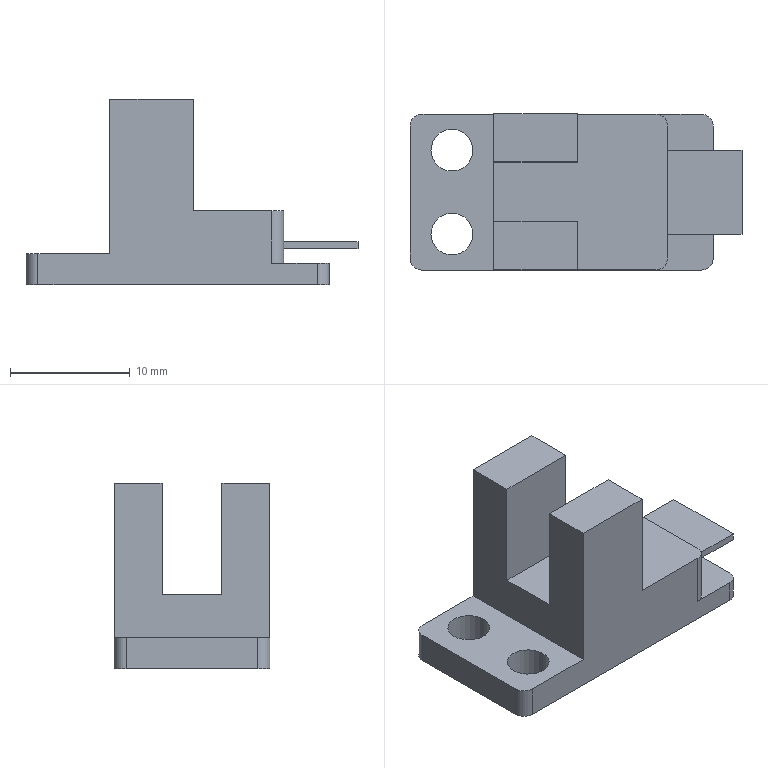Part | NX | 1 solid | 29 faces | box 27.7 x 13 x 15.5 mm | volume 1984 mm3 | plane 21 | cylinder 8 | commonest cylinder face diameters 2 x6 3.5 x2
STEP:
#1=CARTESIAN_POINT('',(5.25,3.,2.6));
#2=VERTEX_POINT('',#1);
#3=CARTESIAN_POINT('',(3.5,3.,2.6));
#4=DIRECTION('',(0.,0.,1.));
#5=DIRECTION('',(1.,0.,0.));
#6=AXIS2_PLACEMENT_3D('',#3,#4,#5);
#7=CIRCLE('',#6,1.75);
#8=EDGE_CURVE('',#2,#2,#7,.T.);
#9=ORIENTED_EDGE('',*,*,#8,.T.);
#10=EDGE_LOOP('',(#9));
#11=FACE_BOUND('',#10,.T.);
#12=CARTESIAN_POINT('',(5.25,3.,0.));
#13=VERTEX_POINT('',#12);
#14=CARTESIAN_POINT('',(3.5,3.,0.));
#15=DIRECTION('',(0.,0.,1.));
#16=DIRECTION('',(1.,0.,0.));
#17=AXIS2_PLACEMENT_3D('',#14,#15,#16);
#18=CIRCLE('',#17,1.75);
#19=EDGE_CURVE('',#13,#13,#18,.F.);
#20=ORIENTED_EDGE('',*,*,#19,.T.);
#21=EDGE_LOOP('',(#20));
#22=FACE_BOUND('',#21,.T.);
#23=CARTESIAN_POINT('',(3.5,3.,0.));
#24=DIRECTION('',(0.,0.,1.));
#25=DIRECTION('',(1.,0.,0.));
#26=AXIS2_PLACEMENT_3D('',#23,#24,#25);
#27=CYLINDRICAL_SURFACE('',#26,1.75);
#28=ADVANCED_FACE('',(#11,#22),#27,.F.);
#29=CARTESIAN_POINT('',(5.25,10.,2.6));
#30=VERTEX_POINT('',#29);
#31=CARTESIAN_POINT('',(3.5,10.,2.6));
#32=DIRECTION('',(0.,0.,1.));
#33=DIRECTION('',(1.,0.,0.));
#34=AXIS2_PLACEMENT_3D('',#31,#32,#33);
#35=CIRCLE('',#34,1.75);
#36=EDGE_CURVE('',#30,#30,#35,.T.);
#37=ORIENTED_EDGE('',*,*,#36,.F.);
#38=EDGE_LOOP('',(#37));
#39=FACE_BOUND('',#38,.T.);
#40=ORIENTED_EDGE('',*,*,#8,.F.);
#41=EDGE_LOOP('',(#40));
#42=FACE_BOUND('',#41,.T.);
#43=CARTESIAN_POINT('',(0.,1.,2.6));
#44=VERTEX_POINT('',#43);
#45=CARTESIAN_POINT('',(1.,0.,2.6));
#46=VERTEX_POINT('',#45);
#47=CARTESIAN_POINT('',(1.,1.,2.6));
#48=DIRECTION('',(0.,0.,-1.));
#49=DIRECTION('',(-1.,0.,0.));
#50=AXIS2_PLACEMENT_3D('',#47,#48,#49);
#51=CIRCLE('',#50,1.);
#52=EDGE_CURVE('',#44,#46,#51,.F.);
#53=ORIENTED_EDGE('',*,*,#52,.T.);
#54=CARTESIAN_POINT('',(7.,0.,2.6));
#55=VERTEX_POINT('',#54);
#56=CARTESIAN_POINT('',(3.5,0.,2.6));
#57=DIRECTION('',(-1.,0.,0.));
#58=VECTOR('',#57,1000.);
#59=LINE('',#56,#58);
#60=EDGE_CURVE('',#55,#46,#59,.T.);
#61=ORIENTED_EDGE('',*,*,#60,.F.);
#62=CARTESIAN_POINT('',(7.,13.,2.6));
#63=VERTEX_POINT('',#62);
#64=CARTESIAN_POINT('',(7.,6.5,2.6));
#65=DIRECTION('',(0.,-1.,0.));
#66=VECTOR('',#65,1000.);
#67=LINE('',#64,#66);
#68=EDGE_CURVE('',#63,#55,#67,.T.);
#69=ORIENTED_EDGE('',*,*,#68,.F.);
#70=CARTESIAN_POINT('',(1.,13.,2.6));
#71=VERTEX_POINT('',#70);
#72=CARTESIAN_POINT('',(3.5,13.,2.6));
#73=DIRECTION('',(1.,0.,0.));
#74=VECTOR('',#73,1000.);
#75=LINE('',#72,#74);
#76=EDGE_CURVE('',#71,#63,#75,.T.);
#77=ORIENTED_EDGE('',*,*,#76,.F.);
#78=CARTESIAN_POINT('',(0.,12.,2.6));
#79=VERTEX_POINT('',#78);
#80=CARTESIAN_POINT('',(1.,12.,2.6));
#81=DIRECTION('',(0.,0.,-1.));
#82=DIRECTION('',(-1.,0.,0.));
#83=AXIS2_PLACEMENT_3D('',#80,#81,#82);
#84=CIRCLE('',#83,1.);
#85=EDGE_CURVE('',#71,#79,#84,.F.);
#86=ORIENTED_EDGE('',*,*,#85,.T.);
#87=CARTESIAN_POINT('',(0.,6.5,2.6));
#88=DIRECTION('',(0.,1.,0.));
#89=VECTOR('',#88,1000.);
#90=LINE('',#87,#89);
#91=EDGE_CURVE('',#44,#79,#90,.T.);
#92=ORIENTED_EDGE('',*,*,#91,.F.);
#93=EDGE_LOOP('',(#53,#61,#69,#77,#86,#92));
#94=FACE_BOUND('',#93,.T.);
#95=CARTESIAN_POINT('',(7.,0.,2.6));
#96=DIRECTION('',(0.,0.,-1.));
#97=DIRECTION('',(-1.,0.,0.));
#98=AXIS2_PLACEMENT_3D('',#95,#96,#97);
#99=PLANE('',#98);
#100=ADVANCED_FACE('',(#39,#42,#94),#99,.F.);
#101=CARTESIAN_POINT('',(5.25,10.,0.));
#102=VERTEX_POINT('',#101);
#103=CARTESIAN_POINT('',(3.5,10.,0.));
#104=DIRECTION('',(0.,0.,1.));
#105=DIRECTION('',(1.,0.,0.));
#106=AXIS2_PLACEMENT_3D('',#103,#104,#105);
#107=CIRCLE('',#106,1.75);
#108=EDGE_CURVE('',#102,#102,#107,.T.);
#109=ORIENTED_EDGE('',*,*,#108,.T.);
#110=EDGE_LOOP('',(#109));
#111=FACE_BOUND('',#110,.T.);
#112=ORIENTED_EDGE('',*,*,#19,.F.);
#113=EDGE_LOOP('',(#112));
#114=FACE_BOUND('',#113,.T.);
#115=CARTESIAN_POINT('',(1.,13.,0.));
#116=VERTEX_POINT('',#115);
#117=CARTESIAN_POINT('',(24.3,13.,0.));
#118=VERTEX_POINT('',#117);
#119=CARTESIAN_POINT('',(12.65,13.,0.));
#120=DIRECTION('',(1.,0.,0.));
#121=VECTOR('',#120,1000.);
#122=LINE('',#119,#121);
#123=EDGE_CURVE('',#116,#118,#122,.T.);
#124=ORIENTED_EDGE('',*,*,#123,.T.);
#125=CARTESIAN_POINT('',(25.3,12.,0.));
#126=VERTEX_POINT('',#125);
#127=CARTESIAN_POINT('',(24.3,12.,0.));
#128=DIRECTION('',(0.,0.,-1.));
#129=DIRECTION('',(-1.,0.,0.));
#130=AXIS2_PLACEMENT_3D('',#127,#128,#129);
#131=CIRCLE('',#130,1.);
#132=EDGE_CURVE('',#118,#126,#131,.T.);
#133=ORIENTED_EDGE('',*,*,#132,.T.);
#134=CARTESIAN_POINT('',(25.3,1.,0.));
#135=VERTEX_POINT('',#134);
#136=CARTESIAN_POINT('',(25.3,6.5,0.));
#137=DIRECTION('',(0.,-1.,0.));
#138=VECTOR('',#137,1000.);
#139=LINE('',#136,#138);
#140=EDGE_CURVE('',#126,#135,#139,.T.);
#141=ORIENTED_EDGE('',*,*,#140,.T.);
#142=CARTESIAN_POINT('',(24.3,0.,0.));
#143=VERTEX_POINT('',#142);
#144=CARTESIAN_POINT('',(24.3,1.,0.));
#145=DIRECTION('',(0.,0.,-1.));
#146=DIRECTION('',(-1.,0.,0.));
#147=AXIS2_PLACEMENT_3D('',#144,#145,#146);
#148=CIRCLE('',#147,1.);
#149=EDGE_CURVE('',#135,#143,#148,.T.);
#150=ORIENTED_EDGE('',*,*,#149,.T.);
#151=CARTESIAN_POINT('',(1.,0.,0.));
#152=VERTEX_POINT('',#151);
#153=CARTESIAN_POINT('',(12.65,0.,0.));
#154=DIRECTION('',(-1.,0.,0.));
#155=VECTOR('',#154,1000.);
#156=LINE('',#153,#155);
#157=EDGE_CURVE('',#143,#152,#156,.T.);
#158=ORIENTED_EDGE('',*,*,#157,.T.);
#159=CARTESIAN_POINT('',(0.,1.,0.));
#160=VERTEX_POINT('',#159);
#161=CARTESIAN_POINT('',(1.,1.,0.));
#162=DIRECTION('',(0.,0.,-1.));
#163=DIRECTION('',(-1.,0.,0.));
#164=AXIS2_PLACEMENT_3D('',#161,#162,#163);
#165=CIRCLE('',#164,1.);
#166=EDGE_CURVE('',#152,#160,#165,.T.);
#167=ORIENTED_EDGE('',*,*,#166,.T.);
#168=CARTESIAN_POINT('',(0.,12.,0.));
#169=VERTEX_POINT('',#168);
#170=CARTESIAN_POINT('',(0.,6.5,0.));
#171=DIRECTION('',(0.,1.,0.));
#172=VECTOR('',#171,1000.);
#173=LINE('',#170,#172);
#174=EDGE_CURVE('',#160,#169,#173,.T.);
#175=ORIENTED_EDGE('',*,*,#174,.T.);
#176=CARTESIAN_POINT('',(1.,12.,0.));
#177=DIRECTION('',(0.,0.,-1.));
#178=DIRECTION('',(-1.,0.,0.));
#179=AXIS2_PLACEMENT_3D('',#176,#177,#178);
#180=CIRCLE('',#179,1.);
#181=EDGE_CURVE('',#169,#116,#180,.T.);
#182=ORIENTED_EDGE('',*,*,#181,.T.);
#183=EDGE_LOOP('',(#124,#133,#141,#150,#158,#167,#175,#182));
#184=FACE_BOUND('',#183,.T.);
#185=CARTESIAN_POINT('',(25.3,0.,0.));
#186=DIRECTION('',(0.,0.,-1.));
#187=DIRECTION('',(-1.,0.,0.));
#188=AXIS2_PLACEMENT_3D('',#185,#186,#187);
#189=PLANE('',#188);
#190=ADVANCED_FACE('',(#111,#114,#184),#189,.T.);
#191=ORIENTED_EDGE('',*,*,#108,.F.);
#192=EDGE_LOOP('',(#191));
#193=FACE_BOUND('',#192,.T.);
#194=ORIENTED_EDGE('',*,*,#36,.T.);
#195=EDGE_LOOP('',(#194));
#196=FACE_BOUND('',#195,.T.);
#197=CARTESIAN_POINT('',(3.5,10.,0.));
#198=DIRECTION('',(0.,0.,1.));
#199=DIRECTION('',(1.,0.,0.));
#200=AXIS2_PLACEMENT_3D('',#197,#198,#199);
#201=CYLINDRICAL_SURFACE('',#200,1.75);
#202=ADVANCED_FACE('',(#193,#196),#201,.F.);
#203=CARTESIAN_POINT('',(0.,1.,1.3));
#204=DIRECTION('',(0.,0.,-1.));
#205=VECTOR('',#204,1000.);
#206=LINE('',#203,#205);
#207=EDGE_CURVE('',#44,#160,#206,.T.);
#208=ORIENTED_EDGE('',*,*,#207,.F.);
#209=ORIENTED_EDGE('',*,*,#91,.T.);
#210=CARTESIAN_POINT('',(0.,12.,1.3));
#211=DIRECTION('',(0.,0.,1.));
#212=VECTOR('',#211,1000.);
#213=LINE('',#210,#212);
#214=EDGE_CURVE('',#169,#79,#213,.T.);
#215=ORIENTED_EDGE('',*,*,#214,.F.);
#216=ORIENTED_EDGE('',*,*,#174,.F.);
#217=EDGE_LOOP('',(#208,#209,#215,#216));
#218=FACE_BOUND('',#217,.T.);
#219=CARTESIAN_POINT('',(0.,1.,2.6));
#220=DIRECTION('',(1.,0.,0.));
#221=DIRECTION('',(0.,0.,-1.));
#222=AXIS2_PLACEMENT_3D('',#219,#220,#221);
#223=PLANE('',#222);
#224=ADVANCED_FACE('',(#218),#223,.F.);
#225=CARTESIAN_POINT('',(24.3,0.,1.8));
#226=VERTEX_POINT('',#225);
#227=CARTESIAN_POINT('',(24.3,0.,7.75));
#228=DIRECTION('',(0.,0.,-1.));
#229=VECTOR('',#228,1000.);
#230=LINE('',#227,#229);
#231=EDGE_CURVE('',#226,#143,#230,.T.);
#232=ORIENTED_EDGE('',*,*,#231,.F.);
#233=CARTESIAN_POINT('',(20.5,0.,1.8));
#234=VERTEX_POINT('',#233);
#235=CARTESIAN_POINT('',(12.65,0.,1.8));
#236=DIRECTION('',(1.,0.,0.));
#237=VECTOR('',#236,1000.);
#238=LINE('',#235,#237);
#239=EDGE_CURVE('',#234,#226,#238,.T.);
#240=ORIENTED_EDGE('',*,*,#239,.F.);
#241=CARTESIAN_POINT('',(20.5,0.,6.2));
#242=VERTEX_POINT('',#241);
#243=CARTESIAN_POINT('',(20.5,0.,7.75));
#244=DIRECTION('',(0.,0.,-1.));
#245=VECTOR('',#244,1000.);
#246=LINE('',#243,#245);
#247=EDGE_CURVE('',#242,#234,#246,.T.);
#248=ORIENTED_EDGE('',*,*,#247,.F.);
#249=CARTESIAN_POINT('',(13.95,0.,6.2));
#250=VERTEX_POINT('',#249);
#251=CARTESIAN_POINT('',(12.65,0.,6.2));
#252=DIRECTION('',(1.,0.,0.));
#253=VECTOR('',#252,1000.);
#254=LINE('',#251,#253);
#255=EDGE_CURVE('',#250,#242,#254,.T.);
#256=ORIENTED_EDGE('',*,*,#255,.F.);
#257=CARTESIAN_POINT('',(13.95,0.,15.5));
#258=VERTEX_POINT('',#257);
#259=CARTESIAN_POINT('',(13.95,0.,7.75));
#260=DIRECTION('',(0.,0.,-1.));
#261=VECTOR('',#260,1000.);
#262=LINE('',#259,#261);
#263=EDGE_CURVE('',#258,#250,#262,.T.);
#264=ORIENTED_EDGE('',*,*,#263,.F.);
#265=CARTESIAN_POINT('',(7.,0.,15.5));
#266=VERTEX_POINT('',#265);
#267=CARTESIAN_POINT('',(12.65,0.,15.5));
#268=DIRECTION('',(1.,0.,0.));
#269=VECTOR('',#268,1000.);
#270=LINE('',#267,#269);
#271=EDGE_CURVE('',#266,#258,#270,.T.);
#272=ORIENTED_EDGE('',*,*,#271,.F.);
#273=CARTESIAN_POINT('',(7.,0.,7.75));
#274=DIRECTION('',(0.,0.,1.));
#275=VECTOR('',#274,1000.);
#276=LINE('',#273,#275);
#277=EDGE_CURVE('',#55,#266,#276,.T.);
#278=ORIENTED_EDGE('',*,*,#277,.F.);
#279=ORIENTED_EDGE('',*,*,#60,.T.);
#280=CARTESIAN_POINT('',(1.,0.,7.75));
#281=DIRECTION('',(0.,0.,1.));
#282=VECTOR('',#281,1000.);
#283=LINE('',#280,#282);
#284=EDGE_CURVE('',#152,#46,#283,.T.);
#285=ORIENTED_EDGE('',*,*,#284,.F.);
#286=ORIENTED_EDGE('',*,*,#157,.F.);
#287=EDGE_LOOP('',(#232,#240,#248,#256,#264,#272,#278,#279,#285,#286));
#288=FACE_BOUND('',#287,.T.);
#289=CARTESIAN_POINT('',(1.,0.,0.));
#290=DIRECTION('',(0.,1.,0.));
#291=DIRECTION('',(0.,0.,1.));
#292=AXIS2_PLACEMENT_3D('',#289,#290,#291);
#293=PLANE('',#292);
#294=ADVANCED_FACE('',(#288),#293,.F.);
#295=CARTESIAN_POINT('',(7.,4.,6.2));
#296=VERTEX_POINT('',#295);
#297=CARTESIAN_POINT('',(7.,4.,15.5));
#298=VERTEX_POINT('',#297);
#299=CARTESIAN_POINT('',(7.,4.,9.05));
#300=DIRECTION('',(0.,0.,1.));
#301=VECTOR('',#300,1000.);
#302=LINE('',#299,#301);
#303=EDGE_CURVE('',#296,#298,#302,.T.);
#304=ORIENTED_EDGE('',*,*,#303,.F.);
#305=CARTESIAN_POINT('',(7.,9.,6.2));
#306=VERTEX_POINT('',#305);
#307=CARTESIAN_POINT('',(7.,6.5,6.2));
#308=DIRECTION('',(0.,-1.,0.));
#309=VECTOR('',#308,1000.);
#310=LINE('',#307,#309);
#311=EDGE_CURVE('',#306,#296,#310,.T.);
#312=ORIENTED_EDGE('',*,*,#311,.F.);
#313=CARTESIAN_POINT('',(7.,9.,15.5));
#314=VERTEX_POINT('',#313);
#315=CARTESIAN_POINT('',(7.,9.,9.05));
#316=DIRECTION('',(0.,0.,-1.));
#317=VECTOR('',#316,1000.);
#318=LINE('',#315,#317);
#319=EDGE_CURVE('',#314,#306,#318,.T.);
#320=ORIENTED_EDGE('',*,*,#319,.F.);
#321=CARTESIAN_POINT('',(7.,13.,15.5));
#322=VERTEX_POINT('',#321);
#323=CARTESIAN_POINT('',(7.,6.5,15.5));
#324=DIRECTION('',(0.,-1.,0.));
#325=VECTOR('',#324,1000.);
#326=LINE('',#323,#325);
#327=EDGE_CURVE('',#322,#314,#326,.T.);
#328=ORIENTED_EDGE('',*,*,#327,.F.);
#329=CARTESIAN_POINT('',(7.,13.,9.05));
#330=DIRECTION('',(0.,0.,1.));
#331=VECTOR('',#330,1000.);
#332=LINE('',#329,#331);
#333=EDGE_CURVE('',#63,#322,#332,.T.);
#334=ORIENTED_EDGE('',*,*,#333,.F.);
#335=ORIENTED_EDGE('',*,*,#68,.T.);
#336=ORIENTED_EDGE('',*,*,#277,.T.);
#337=CARTESIAN_POINT('',(7.,6.5,15.5));
#338=DIRECTION('',(0.,-1.,0.));
#339=VECTOR('',#338,1000.);
#340=LINE('',#337,#339);
#341=EDGE_CURVE('',#298,#266,#340,.T.);
#342=ORIENTED_EDGE('',*,*,#341,.F.);
#343=EDGE_LOOP('',(#304,#312,#320,#328,#334,#335,#336,#342));
#344=FACE_BOUND('',#343,.T.);
#345=CARTESIAN_POINT('',(7.,0.,15.5));
#346=DIRECTION('',(1.,0.,0.));
#347=DIRECTION('',(0.,0.,-1.));
#348=AXIS2_PLACEMENT_3D('',#345,#346,#347);
#349=PLANE('',#348);
#350=ADVANCED_FACE('',(#344),#349,.F.);
#351=CARTESIAN_POINT('',(24.3,13.,1.8));
#352=VERTEX_POINT('',#351);
#353=CARTESIAN_POINT('',(24.3,13.,7.75));
#354=DIRECTION('',(0.,0.,1.));
#355=VECTOR('',#354,1000.);
#356=LINE('',#353,#355);
#357=EDGE_CURVE('',#118,#352,#356,.T.);
#358=ORIENTED_EDGE('',*,*,#357,.F.);
#359=ORIENTED_EDGE('',*,*,#123,.F.);
#360=CARTESIAN_POINT('',(1.,13.,7.75));
#361=DIRECTION('',(0.,0.,-1.));
#362=VECTOR('',#361,1000.);
#363=LINE('',#360,#362);
#364=EDGE_CURVE('',#71,#116,#363,.T.);
#365=ORIENTED_EDGE('',*,*,#364,.F.);
#366=ORIENTED_EDGE('',*,*,#76,.T.);
#367=ORIENTED_EDGE('',*,*,#333,.T.);
#368=CARTESIAN_POINT('',(13.95,13.,15.5));
#369=VERTEX_POINT('',#368);
#370=CARTESIAN_POINT('',(12.65,13.,15.5));
#371=DIRECTION('',(-1.,0.,0.));
#372=VECTOR('',#371,1000.);
#373=LINE('',#370,#372);
#374=EDGE_CURVE('',#369,#322,#373,.T.);
#375=ORIENTED_EDGE('',*,*,#374,.F.);
#376=CARTESIAN_POINT('',(13.95,13.,6.2));
#377=VERTEX_POINT('',#376);
#378=CARTESIAN_POINT('',(13.95,13.,7.75));
#379=DIRECTION('',(0.,0.,1.));
#380=VECTOR('',#379,1000.);
#381=LINE('',#378,#380);
#382=EDGE_CURVE('',#377,#369,#381,.T.);
#383=ORIENTED_EDGE('',*,*,#382,.F.);
#384=CARTESIAN_POINT('',(20.5,13.,6.2));
#385=VERTEX_POINT('',#384);
#386=CARTESIAN_POINT('',(12.65,13.,6.2));
#387=DIRECTION('',(-1.,0.,0.));
#388=VECTOR('',#387,1000.);
#389=LINE('',#386,#388);
#390=EDGE_CURVE('',#385,#377,#389,.T.);
#391=ORIENTED_EDGE('',*,*,#390,.F.);
#392=CARTESIAN_POINT('',(20.5,13.,1.8));
#393=VERTEX_POINT('',#392);
#394=CARTESIAN_POINT('',(20.5,13.,7.75));
#395=DIRECTION('',(0.,0.,1.));
#396=VECTOR('',#395,1000.);
#397=LINE('',#394,#396);
#398=EDGE_CURVE('',#393,#385,#397,.T.);
#399=ORIENTED_EDGE('',*,*,#398,.F.);
#400=CARTESIAN_POINT('',(12.65,13.,1.8));
#401=DIRECTION('',(-1.,0.,0.));
#402=VECTOR('',#401,1000.);
#403=LINE('',#400,#402);
#404=EDGE_CURVE('',#352,#393,#403,.T.);
#405=ORIENTED_EDGE('',*,*,#404,.F.);
#406=EDGE_LOOP('',(#358,#359,#365,#366,#367,#375,#383,#391,#399,#405));
#407=FACE_BOUND('',#406,.T.);
#408=CARTESIAN_POINT('',(1.,13.,15.5));
#409=DIRECTION('',(0.,-1.,0.));
#410=DIRECTION('',(0.,0.,-1.));
#411=AXIS2_PLACEMENT_3D('',#408,#409,#410);
#412=PLANE('',#411);
#413=ADVANCED_FACE('',(#407),#412,.F.);
#414=ORIENTED_EDGE('',*,*,#140,.F.);
#415=CARTESIAN_POINT('',(25.3,12.,1.8));
#416=VERTEX_POINT('',#415);
#417=CARTESIAN_POINT('',(25.3,12.,0.9));
#418=DIRECTION('',(0.,0.,1.));
#419=VECTOR('',#418,1000.);
#420=LINE('',#417,#419);
#421=EDGE_CURVE('',#126,#416,#420,.T.);
#422=ORIENTED_EDGE('',*,*,#421,.T.);
#423=CARTESIAN_POINT('',(25.3,1.,1.8));
#424=VERTEX_POINT('',#423);
#425=CARTESIAN_POINT('',(25.3,6.5,1.8));
#426=DIRECTION('',(0.,-1.,0.));
#427=VECTOR('',#426,1000.);
#428=LINE('',#425,#427);
#429=EDGE_CURVE('',#416,#424,#428,.T.);
#430=ORIENTED_EDGE('',*,*,#429,.T.);
#431=CARTESIAN_POINT('',(25.3,1.,0.9));
#432=DIRECTION('',(0.,0.,-1.));
#433=VECTOR('',#432,1000.);
#434=LINE('',#431,#433);
#435=EDGE_CURVE('',#424,#135,#434,.T.);
#436=ORIENTED_EDGE('',*,*,#435,.T.);
#437=EDGE_LOOP('',(#414,#422,#430,#436));
#438=FACE_BOUND('',#437,.T.);
#439=CARTESIAN_POINT('',(25.3,1.,1.8));
#440=DIRECTION('',(1.,0.,0.));
#441=DIRECTION('',(0.,0.,-1.));
#442=AXIS2_PLACEMENT_3D('',#439,#440,#441);
#443=PLANE('',#442);
#444=ADVANCED_FACE('',(#438),#443,.T.);
#445=ORIENTED_EDGE('',*,*,#207,.T.);
#446=ORIENTED_EDGE('',*,*,#166,.F.);
#447=ORIENTED_EDGE('',*,*,#284,.T.);
#448=ORIENTED_EDGE('',*,*,#52,.F.);
#449=EDGE_LOOP('',(#445,#446,#447,#448));
#450=FACE_BOUND('',#449,.T.);
#451=CARTESIAN_POINT('',(1.,1.,2.6));
#452=DIRECTION('',(0.,0.,-1.));
#453=DIRECTION('',(-1.,0.,0.));
#454=AXIS2_PLACEMENT_3D('',#451,#452,#453);
#455=CYLINDRICAL_SURFACE('',#454,1.);
#456=ADVANCED_FACE('',(#450),#455,.T.);
#457=ORIENTED_EDGE('',*,*,#364,.T.);
#458=ORIENTED_EDGE('',*,*,#181,.F.);
#459=ORIENTED_EDGE('',*,*,#214,.T.);
#460=ORIENTED_EDGE('',*,*,#85,.F.);
#461=EDGE_LOOP('',(#457,#458,#459,#460));
#462=FACE_BOUND('',#461,.T.);
#463=CARTESIAN_POINT('',(1.,12.,2.6));
#464=DIRECTION('',(0.,0.,-1.));
#465=DIRECTION('',(-1.,0.,0.));
#466=AXIS2_PLACEMENT_3D('',#463,#464,#465);
#467=CYLINDRICAL_SURFACE('',#466,1.);
#468=ADVANCED_FACE('',(#462),#467,.T.);
#469=ORIENTED_EDGE('',*,*,#435,.F.);
#470=CARTESIAN_POINT('',(24.3,1.,1.8));
#471=DIRECTION('',(0.,0.,-1.));
#472=DIRECTION('',(-1.,0.,0.));
#473=AXIS2_PLACEMENT_3D('',#470,#471,#472);
#474=CIRCLE('',#473,1.);
#475=EDGE_CURVE('',#226,#424,#474,.F.);
#476=ORIENTED_EDGE('',*,*,#475,.F.);
#477=ORIENTED_EDGE('',*,*,#231,.T.);
#478=ORIENTED_EDGE('',*,*,#149,.F.);
#479=EDGE_LOOP('',(#469,#476,#477,#478));
#480=FACE_BOUND('',#479,.T.);
#481=CARTESIAN_POINT('',(24.3,1.,1.8));
#482=DIRECTION('',(0.,0.,-1.));
#483=DIRECTION('',(-1.,0.,0.));
#484=AXIS2_PLACEMENT_3D('',#481,#482,#483);
#485=CYLINDRICAL_SURFACE('',#484,1.);
#486=ADVANCED_FACE('',(#480),#485,.T.);
#487=ORIENTED_EDGE('',*,*,#475,.T.);
#488=ORIENTED_EDGE('',*,*,#429,.F.);
#489=CARTESIAN_POINT('',(24.3,12.,1.8));
#490=DIRECTION('',(0.,0.,-1.));
#491=DIRECTION('',(-1.,0.,0.));
#492=AXIS2_PLACEMENT_3D('',#489,#490,#491);
#493=CIRCLE('',#492,1.);
#494=EDGE_CURVE('',#352,#416,#493,.T.);
#495=ORIENTED_EDGE('',*,*,#494,.F.);
#496=ORIENTED_EDGE('',*,*,#404,.T.);
#497=CARTESIAN_POINT('',(21.5,12.,1.8));
#498=VERTEX_POINT('',#497);
#499=CARTESIAN_POINT('',(20.5,12.,1.8));
#500=DIRECTION('',(0.,0.,-1.));
#501=DIRECTION('',(-1.,0.,0.));
#502=AXIS2_PLACEMENT_3D('',#499,#500,#501);
#503=CIRCLE('',#502,1.);
#504=EDGE_CURVE('',#498,#393,#503,.F.);
#505=ORIENTED_EDGE('',*,*,#504,.F.);
#506=CARTESIAN_POINT('',(21.5,1.,1.8));
#507=VERTEX_POINT('',#506);
#508=CARTESIAN_POINT('',(21.5,6.5,1.8));
#509=DIRECTION('',(0.,1.,0.));
#510=VECTOR('',#509,1000.);
#511=LINE('',#508,#510);
#512=EDGE_CURVE('',#507,#498,#511,.T.);
#513=ORIENTED_EDGE('',*,*,#512,.F.);
#514=CARTESIAN_POINT('',(20.5,1.,1.8));
#515=DIRECTION('',(0.,0.,-1.));
#516=DIRECTION('',(-1.,0.,0.));
#517=AXIS2_PLACEMENT_3D('',#514,#515,#516);
#518=CIRCLE('',#517,1.);
#519=EDGE_CURVE('',#234,#507,#518,.F.);
#520=ORIENTED_EDGE('',*,*,#519,.F.);
#521=ORIENTED_EDGE('',*,*,#239,.T.);
#522=EDGE_LOOP('',(#487,#488,#495,#496,#505,#513,#520,#521));
#523=FACE_BOUND('',#522,.T.);
#524=CARTESIAN_POINT('',(20.471,0.,1.8));
#525=DIRECTION('',(0.,0.,-1.));
#526=DIRECTION('',(0.,1.,0.));
#527=AXIS2_PLACEMENT_3D('',#524,#525,#526);
#528=PLANE('',#527);
#529=ADVANCED_FACE('',(#523),#528,.F.);
#530=ORIENTED_EDGE('',*,*,#247,.T.);
#531=ORIENTED_EDGE('',*,*,#519,.T.);
#532=CARTESIAN_POINT('',(21.5,1.,6.2));
#533=VERTEX_POINT('',#532);
#534=CARTESIAN_POINT('',(21.5,1.,4.));
#535=DIRECTION('',(0.,0.,1.));
#536=VECTOR('',#535,1000.);
#537=LINE('',#534,#536);
#538=EDGE_CURVE('',#533,#507,#537,.F.);
#539=ORIENTED_EDGE('',*,*,#538,.F.);
#540=CARTESIAN_POINT('',(20.5,1.,6.2));
#541=DIRECTION('',(0.,0.,-1.));
#542=DIRECTION('',(-1.,0.,0.));
#543=AXIS2_PLACEMENT_3D('',#540,#541,#542);
#544=CIRCLE('',#543,1.);
#545=EDGE_CURVE('',#242,#533,#544,.F.);
#546=ORIENTED_EDGE('',*,*,#545,.F.);
#547=EDGE_LOOP('',(#530,#531,#539,#546));
#548=FACE_BOUND('',#547,.T.);
#549=CARTESIAN_POINT('',(20.5,1.,6.2));
#550=DIRECTION('',(0.,0.,-1.));
#551=DIRECTION('',(-1.,0.,0.));
#552=AXIS2_PLACEMENT_3D('',#549,#550,#551);
#553=CYLINDRICAL_SURFACE('',#552,1.);
#554=ADVANCED_FACE('',(#548),#553,.T.);
#555=ORIENTED_EDGE('',*,*,#545,.T.);
#556=CARTESIAN_POINT('',(21.5,12.,6.2));
#557=VERTEX_POINT('',#556);
#558=CARTESIAN_POINT('',(21.5,6.5,6.2));
#559=DIRECTION('',(0.,-1.,0.));
#560=VECTOR('',#559,1000.);
#561=LINE('',#558,#560);
#562=EDGE_CURVE('',#557,#533,#561,.T.);
#563=ORIENTED_EDGE('',*,*,#562,.F.);
#564=CARTESIAN_POINT('',(20.5,12.,6.2));
#565=DIRECTION('',(0.,0.,-1.));
#566=DIRECTION('',(-1.,0.,0.));
#567=AXIS2_PLACEMENT_3D('',#564,#565,#566);
#568=CIRCLE('',#567,1.);
#569=EDGE_CURVE('',#385,#557,#568,.T.);
#570=ORIENTED_EDGE('',*,*,#569,.F.);
#571=ORIENTED_EDGE('',*,*,#390,.T.);
#572=CARTESIAN_POINT('',(13.95,9.,6.2));
#573=VERTEX_POINT('',#572);
#574=CARTESIAN_POINT('',(13.95,6.5,6.2));
#575=DIRECTION('',(0.,1.,0.));
#576=VECTOR('',#575,1000.);
#577=LINE('',#574,#576);
#578=EDGE_CURVE('',#573,#377,#577,.T.);
#579=ORIENTED_EDGE('',*,*,#578,.F.);
#580=CARTESIAN_POINT('',(14.25,9.,6.2));
#581=DIRECTION('',(1.,0.,0.));
#582=VECTOR('',#581,1000.);
#583=LINE('',#580,#582);
#584=EDGE_CURVE('',#306,#573,#583,.T.);
#585=ORIENTED_EDGE('',*,*,#584,.F.);
#586=ORIENTED_EDGE('',*,*,#311,.T.);
#587=CARTESIAN_POINT('',(13.95,4.,6.2));
#588=VERTEX_POINT('',#587);
#589=CARTESIAN_POINT('',(14.25,4.,6.2));
#590=DIRECTION('',(-1.,0.,0.));
#591=VECTOR('',#590,1000.);
#592=LINE('',#589,#591);
#593=EDGE_CURVE('',#588,#296,#592,.T.);
#594=ORIENTED_EDGE('',*,*,#593,.F.);
#595=CARTESIAN_POINT('',(13.95,6.5,6.2));
#596=DIRECTION('',(0.,1.,0.));
#597=VECTOR('',#596,1000.);
#598=LINE('',#595,#597);
#599=EDGE_CURVE('',#250,#588,#598,.T.);
#600=ORIENTED_EDGE('',*,*,#599,.F.);
#601=ORIENTED_EDGE('',*,*,#255,.T.);
#602=EDGE_LOOP('',(#555,#563,#570,#571,#579,#585,#586,#594,#600,#601));
#603=FACE_BOUND('',#602,.T.);
#604=CARTESIAN_POINT('',(7.,0.,6.2));
#605=DIRECTION('',(0.,0.,-1.));
#606=DIRECTION('',(0.,1.,0.));
#607=AXIS2_PLACEMENT_3D('',#604,#605,#606);
#608=PLANE('',#607);
#609=ADVANCED_FACE('',(#603),#608,.F.);
#610=ORIENTED_EDGE('',*,*,#263,.T.);
#611=ORIENTED_EDGE('',*,*,#599,.T.);
#612=CARTESIAN_POINT('',(13.95,4.,15.5));
#613=VERTEX_POINT('',#612);
#614=CARTESIAN_POINT('',(13.95,4.,10.85));
#615=DIRECTION('',(0.,0.,-1.));
#616=VECTOR('',#615,1000.);
#617=LINE('',#614,#616);
#618=EDGE_CURVE('',#613,#588,#617,.T.);
#619=ORIENTED_EDGE('',*,*,#618,.F.);
#620=CARTESIAN_POINT('',(13.95,2.,15.5));
#621=DIRECTION('',(0.,1.,0.));
#622=VECTOR('',#621,1000.);
#623=LINE('',#620,#622);
#624=EDGE_CURVE('',#258,#613,#623,.T.);
#625=ORIENTED_EDGE('',*,*,#624,.F.);
#626=EDGE_LOOP('',(#610,#611,#619,#625));
#627=FACE_BOUND('',#626,.T.);
#628=CARTESIAN_POINT('',(13.95,0.,6.2));
#629=DIRECTION('',(-1.,0.,0.));
#630=DIRECTION('',(0.,0.,1.));
#631=AXIS2_PLACEMENT_3D('',#628,#629,#630);
#632=PLANE('',#631);
#633=ADVANCED_FACE('',(#627),#632,.F.);
#634=ORIENTED_EDGE('',*,*,#624,.T.);
#635=CARTESIAN_POINT('',(10.475,4.,15.5));
#636=DIRECTION('',(1.,0.,0.));
#637=VECTOR('',#636,1000.);
#638=LINE('',#635,#637);
#639=EDGE_CURVE('',#298,#613,#638,.T.);
#640=ORIENTED_EDGE('',*,*,#639,.F.);
#641=ORIENTED_EDGE('',*,*,#341,.T.);
#642=ORIENTED_EDGE('',*,*,#271,.T.);
#643=EDGE_LOOP('',(#634,#640,#641,#642));
#644=FACE_BOUND('',#643,.T.);
#645=CARTESIAN_POINT('',(13.95,0.,15.5));
#646=DIRECTION('',(0.,0.,-1.));
#647=DIRECTION('',(-1.,0.,0.));
#648=AXIS2_PLACEMENT_3D('',#645,#646,#647);
#649=PLANE('',#648);
#650=ADVANCED_FACE('',(#644),#649,.F.);
#651=ORIENTED_EDGE('',*,*,#618,.T.);
#652=ORIENTED_EDGE('',*,*,#593,.T.);
#653=ORIENTED_EDGE('',*,*,#303,.T.);
#654=ORIENTED_EDGE('',*,*,#639,.T.);
#655=EDGE_LOOP('',(#651,#652,#653,#654));
#656=FACE_BOUND('',#655,.T.);
#657=CARTESIAN_POINT('',(7.,4.,15.5));
#658=DIRECTION('',(0.,-1.,0.));
#659=DIRECTION('',(0.,0.,-1.));
#660=AXIS2_PLACEMENT_3D('',#657,#658,#659);
#661=PLANE('',#660);
#662=ADVANCED_FACE('',(#656),#661,.F.);
#663=CARTESIAN_POINT('',(13.95,9.,15.5));
#664=VERTEX_POINT('',#663);
#665=CARTESIAN_POINT('',(13.95,9.,10.85));
#666=DIRECTION('',(0.,0.,-1.));
#667=VECTOR('',#666,1000.);
#668=LINE('',#665,#667);
#669=EDGE_CURVE('',#664,#573,#668,.T.);
#670=ORIENTED_EDGE('',*,*,#669,.F.);
#671=CARTESIAN_POINT('',(10.475,9.,15.5));
#672=DIRECTION('',(1.,0.,0.));
#673=VECTOR('',#672,1000.);
#674=LINE('',#671,#673);
#675=EDGE_CURVE('',#314,#664,#674,.T.);
#676=ORIENTED_EDGE('',*,*,#675,.F.);
#677=ORIENTED_EDGE('',*,*,#319,.T.);
#678=ORIENTED_EDGE('',*,*,#584,.T.);
#679=EDGE_LOOP('',(#670,#676,#677,#678));
#680=FACE_BOUND('',#679,.T.);
#681=CARTESIAN_POINT('',(7.,9.,6.2));
#682=DIRECTION('',(0.,1.,0.));
#683=DIRECTION('',(0.,0.,1.));
#684=AXIS2_PLACEMENT_3D('',#681,#682,#683);
#685=PLANE('',#684);
#686=ADVANCED_FACE('',(#680),#685,.F.);
#687=CARTESIAN_POINT('',(13.95,11.,15.5));
#688=DIRECTION('',(0.,-1.,0.));
#689=VECTOR('',#688,1000.);
#690=LINE('',#687,#689);
#691=EDGE_CURVE('',#369,#664,#690,.T.);
#692=ORIENTED_EDGE('',*,*,#691,.F.);
#693=ORIENTED_EDGE('',*,*,#374,.T.);
#694=ORIENTED_EDGE('',*,*,#327,.T.);
#695=ORIENTED_EDGE('',*,*,#675,.T.);
#696=EDGE_LOOP('',(#692,#693,#694,#695));
#697=FACE_BOUND('',#696,.T.);
#698=CARTESIAN_POINT('',(13.95,9.,15.5));
#699=DIRECTION('',(0.,0.,-1.));
#700=DIRECTION('',(-1.,0.,0.));
#701=AXIS2_PLACEMENT_3D('',#698,#699,#700);
#702=PLANE('',#701);
#703=ADVANCED_FACE('',(#697),#702,.F.);
#704=ORIENTED_EDGE('',*,*,#357,.T.);
#705=ORIENTED_EDGE('',*,*,#494,.T.);
#706=ORIENTED_EDGE('',*,*,#421,.F.);
#707=ORIENTED_EDGE('',*,*,#132,.F.);
#708=EDGE_LOOP('',(#704,#705,#706,#707));
#709=FACE_BOUND('',#708,.T.);
#710=CARTESIAN_POINT('',(24.3,12.,1.8));
#711=DIRECTION('',(0.,0.,-1.));
#712=DIRECTION('',(-1.,0.,0.));
#713=AXIS2_PLACEMENT_3D('',#710,#711,#712);
#714=CYLINDRICAL_SURFACE('',#713,1.);
#715=ADVANCED_FACE('',(#709),#714,.T.);
#716=ORIENTED_EDGE('',*,*,#382,.T.);
#717=ORIENTED_EDGE('',*,*,#691,.T.);
#718=ORIENTED_EDGE('',*,*,#669,.T.);
#719=ORIENTED_EDGE('',*,*,#578,.T.);
#720=EDGE_LOOP('',(#716,#717,#718,#719));
#721=FACE_BOUND('',#720,.T.);
#722=CARTESIAN_POINT('',(13.95,9.,6.2));
#723=DIRECTION('',(-1.,0.,0.));
#724=DIRECTION('',(0.,0.,1.));
#725=AXIS2_PLACEMENT_3D('',#722,#723,#724);
#726=PLANE('',#725);
#727=ADVANCED_FACE('',(#721),#726,.F.);
#728=CARTESIAN_POINT('',(21.5,12.,4.));
#729=DIRECTION('',(0.,0.,-1.));
#730=VECTOR('',#729,1000.);
#731=LINE('',#728,#730);
#732=EDGE_CURVE('',#498,#557,#731,.F.);
#733=ORIENTED_EDGE('',*,*,#732,.F.);
#734=ORIENTED_EDGE('',*,*,#504,.T.);
#735=ORIENTED_EDGE('',*,*,#398,.T.);
#736=ORIENTED_EDGE('',*,*,#569,.T.);
#737=EDGE_LOOP('',(#733,#734,#735,#736));
#738=FACE_BOUND('',#737,.T.);
#739=CARTESIAN_POINT('',(20.5,12.,6.2));
#740=DIRECTION('',(0.,0.,-1.));
#741=DIRECTION('',(-1.,0.,0.));
#742=AXIS2_PLACEMENT_3D('',#739,#740,#741);
#743=CYLINDRICAL_SURFACE('',#742,1.);
#744=ADVANCED_FACE('',(#738),#743,.T.);
#745=CARTESIAN_POINT('',(21.5,10.,3.6));
#746=VERTEX_POINT('',#745);
#747=CARTESIAN_POINT('',(21.5,10.,3.));
#748=VERTEX_POINT('',#747);
#749=CARTESIAN_POINT('',(21.5,10.,3.3));
#750=DIRECTION('',(0.,0.,-1.));
#751=VECTOR('',#750,1000.);
#752=LINE('',#749,#751);
#753=EDGE_CURVE('',#746,#748,#752,.T.);
#754=ORIENTED_EDGE('',*,*,#753,.T.);
#755=CARTESIAN_POINT('',(21.5,3.,3.));
#756=VERTEX_POINT('',#755);
#757=CARTESIAN_POINT('',(21.5,6.5,3.));
#758=DIRECTION('',(0.,1.,0.));
#759=VECTOR('',#758,1000.);
#760=LINE('',#757,#759);
#761=EDGE_CURVE('',#756,#748,#760,.T.);
#762=ORIENTED_EDGE('',*,*,#761,.F.);
#763=CARTESIAN_POINT('',(21.5,3.,3.6));
#764=VERTEX_POINT('',#763);
#765=CARTESIAN_POINT('',(21.5,3.,3.3));
#766=DIRECTION('',(0.,0.,1.));
#767=VECTOR('',#766,1000.);
#768=LINE('',#765,#767);
#769=EDGE_CURVE('',#756,#764,#768,.T.);
#770=ORIENTED_EDGE('',*,*,#769,.T.);
#771=CARTESIAN_POINT('',(21.5,6.5,3.6));
#772=DIRECTION('',(0.,-1.,0.));
#773=VECTOR('',#772,1000.);
#774=LINE('',#771,#773);
#775=EDGE_CURVE('',#746,#764,#774,.T.);
#776=ORIENTED_EDGE('',*,*,#775,.F.);
#777=EDGE_LOOP('',(#754,#762,#770,#776));
#778=FACE_BOUND('',#777,.T.);
#779=ORIENTED_EDGE('',*,*,#538,.T.);
#780=ORIENTED_EDGE('',*,*,#512,.T.);
#781=ORIENTED_EDGE('',*,*,#732,.T.);
#782=ORIENTED_EDGE('',*,*,#562,.T.);
#783=EDGE_LOOP('',(#779,#780,#781,#782));
#784=FACE_BOUND('',#783,.T.);
#785=CARTESIAN_POINT('',(21.5,1.,1.8));
#786=DIRECTION('',(-1.,0.,0.));
#787=DIRECTION('',(0.,0.,1.));
#788=AXIS2_PLACEMENT_3D('',#785,#786,#787);
#789=PLANE('',#788);
#790=ADVANCED_FACE('',(#778,#784),#789,.F.);
#791=CARTESIAN_POINT('',(27.7,3.,3.6));
#792=VERTEX_POINT('',#791);
#793=CARTESIAN_POINT('',(24.6,3.,3.6));
#794=DIRECTION('',(-1.,0.,0.));
#795=VECTOR('',#794,1000.);
#796=LINE('',#793,#795);
#797=EDGE_CURVE('',#792,#764,#796,.T.);
#798=ORIENTED_EDGE('',*,*,#797,.F.);
#799=CARTESIAN_POINT('',(27.7,10.,3.6));
#800=VERTEX_POINT('',#799);
#801=CARTESIAN_POINT('',(27.7,6.5,3.6));
#802=DIRECTION('',(0.,-1.,0.));
#803=VECTOR('',#802,1000.);
#804=LINE('',#801,#803);
#805=EDGE_CURVE('',#800,#792,#804,.T.);
#806=ORIENTED_EDGE('',*,*,#805,.F.);
#807=CARTESIAN_POINT('',(24.6,10.,3.6));
#808=DIRECTION('',(1.,0.,0.));
#809=VECTOR('',#808,1000.);
#810=LINE('',#807,#809);
#811=EDGE_CURVE('',#746,#800,#810,.T.);
#812=ORIENTED_EDGE('',*,*,#811,.F.);
#813=ORIENTED_EDGE('',*,*,#775,.T.);
#814=EDGE_LOOP('',(#798,#806,#812,#813));
#815=FACE_BOUND('',#814,.T.);
#816=CARTESIAN_POINT('',(21.5,3.,3.6));
#817=DIRECTION('',(0.,0.,-1.));
#818=DIRECTION('',(0.,1.,0.));
#819=AXIS2_PLACEMENT_3D('',#816,#817,#818);
#820=PLANE('',#819);
#821=ADVANCED_FACE('',(#815),#820,.F.);
#822=CARTESIAN_POINT('',(27.7,10.,3.));
#823=VERTEX_POINT('',#822);
#824=CARTESIAN_POINT('',(24.6,10.,3.));
#825=DIRECTION('',(-1.,0.,0.));
#826=VECTOR('',#825,1000.);
#827=LINE('',#824,#826);
#828=EDGE_CURVE('',#823,#748,#827,.T.);
#829=ORIENTED_EDGE('',*,*,#828,.F.);
#830=CARTESIAN_POINT('',(27.7,3.,3.));
#831=VERTEX_POINT('',#830);
#832=CARTESIAN_POINT('',(27.7,6.5,3.));
#833=DIRECTION('',(0.,1.,0.));
#834=VECTOR('',#833,1000.);
#835=LINE('',#832,#834);
#836=EDGE_CURVE('',#831,#823,#835,.T.);
#837=ORIENTED_EDGE('',*,*,#836,.F.);
#838=CARTESIAN_POINT('',(24.6,3.,3.));
#839=DIRECTION('',(1.,0.,0.));
#840=VECTOR('',#839,1000.);
#841=LINE('',#838,#840);
#842=EDGE_CURVE('',#756,#831,#841,.T.);
#843=ORIENTED_EDGE('',*,*,#842,.F.);
#844=ORIENTED_EDGE('',*,*,#761,.T.);
#845=EDGE_LOOP('',(#829,#837,#843,#844));
#846=FACE_BOUND('',#845,.T.);
#847=CARTESIAN_POINT('',(21.5,10.,3.));
#848=DIRECTION('',(0.,0.,1.));
#849=DIRECTION('',(0.,-1.,0.));
#850=AXIS2_PLACEMENT_3D('',#847,#848,#849);
#851=PLANE('',#850);
#852=ADVANCED_FACE('',(#846),#851,.F.);
#853=ORIENTED_EDGE('',*,*,#842,.T.);
#854=CARTESIAN_POINT('',(27.7,3.,3.3));
#855=DIRECTION('',(0.,0.,-1.));
#856=VECTOR('',#855,1000.);
#857=LINE('',#854,#856);
#858=EDGE_CURVE('',#792,#831,#857,.T.);
#859=ORIENTED_EDGE('',*,*,#858,.F.);
#860=ORIENTED_EDGE('',*,*,#797,.T.);
#861=ORIENTED_EDGE('',*,*,#769,.F.);
#862=EDGE_LOOP('',(#853,#859,#860,#861));
#863=FACE_BOUND('',#862,.T.);
#864=CARTESIAN_POINT('',(21.5,3.,3.));
#865=DIRECTION('',(0.,1.,0.));
#866=DIRECTION('',(0.,0.,1.));
#867=AXIS2_PLACEMENT_3D('',#864,#865,#866);
#868=PLANE('',#867);
#869=ADVANCED_FACE('',(#863),#868,.F.);
#870=ORIENTED_EDGE('',*,*,#836,.T.);
#871=CARTESIAN_POINT('',(27.7,10.,3.3));
#872=DIRECTION('',(0.,0.,1.));
#873=VECTOR('',#872,1000.);
#874=LINE('',#871,#873);
#875=EDGE_CURVE('',#823,#800,#874,.T.);
#876=ORIENTED_EDGE('',*,*,#875,.T.);
#877=ORIENTED_EDGE('',*,*,#805,.T.);
#878=ORIENTED_EDGE('',*,*,#858,.T.);
#879=EDGE_LOOP('',(#870,#876,#877,#878));
#880=FACE_BOUND('',#879,.T.);
#881=CARTESIAN_POINT('',(27.7,3.,3.6));
#882=DIRECTION('',(1.,0.,0.));
#883=DIRECTION('',(0.,0.,-1.));
#884=AXIS2_PLACEMENT_3D('',#881,#882,#883);
#885=PLANE('',#884);
#886=ADVANCED_FACE('',(#880),#885,.T.);
#887=ORIENTED_EDGE('',*,*,#811,.T.);
#888=ORIENTED_EDGE('',*,*,#875,.F.);
#889=ORIENTED_EDGE('',*,*,#828,.T.);
#890=ORIENTED_EDGE('',*,*,#753,.F.);
#891=EDGE_LOOP('',(#887,#888,#889,#890));
#892=FACE_BOUND('',#891,.T.);
#893=CARTESIAN_POINT('',(21.5,10.,3.6));
#894=DIRECTION('',(0.,-1.,0.));
#895=DIRECTION('',(0.,0.,-1.));
#896=AXIS2_PLACEMENT_3D('',#893,#894,#895);
#897=PLANE('',#896);
#898=ADVANCED_FACE('',(#892),#897,.F.);
#899=CLOSED_SHELL('',(#28,#100,#190,#202,#224,#294,#350,#413,#444,#456,#468,#486,#529,#554,#609,#633,#650,#662,#686,#703,#715,#727,#744,#790,#821,#852,#869,#886,#898));
#900=MANIFOLD_SOLID_BREP('',#899);
#901=(LENGTH_UNIT()NAMED_UNIT(*)SI_UNIT(.MILLI.,.METRE.));
#902=UNCERTAINTY_MEASURE_WITH_UNIT(LENGTH_MEASURE(0.00001),#901,'','');
#903=(NAMED_UNIT(*)PLANE_ANGLE_UNIT()SI_UNIT($,.RADIAN.));
#904=(NAMED_UNIT(*)SI_UNIT($,.STERADIAN.)SOLID_ANGLE_UNIT());
#905=(GEOMETRIC_REPRESENTATION_CONTEXT(3)GLOBAL_UNCERTAINTY_ASSIGNED_CONTEXT((#902))GLOBAL_UNIT_ASSIGNED_CONTEXT((#901,#903,#904))REPRESENTATION_CONTEXT('',''));
#906=ADVANCED_BREP_SHAPE_REPRESENTATION('',(#900),#905);